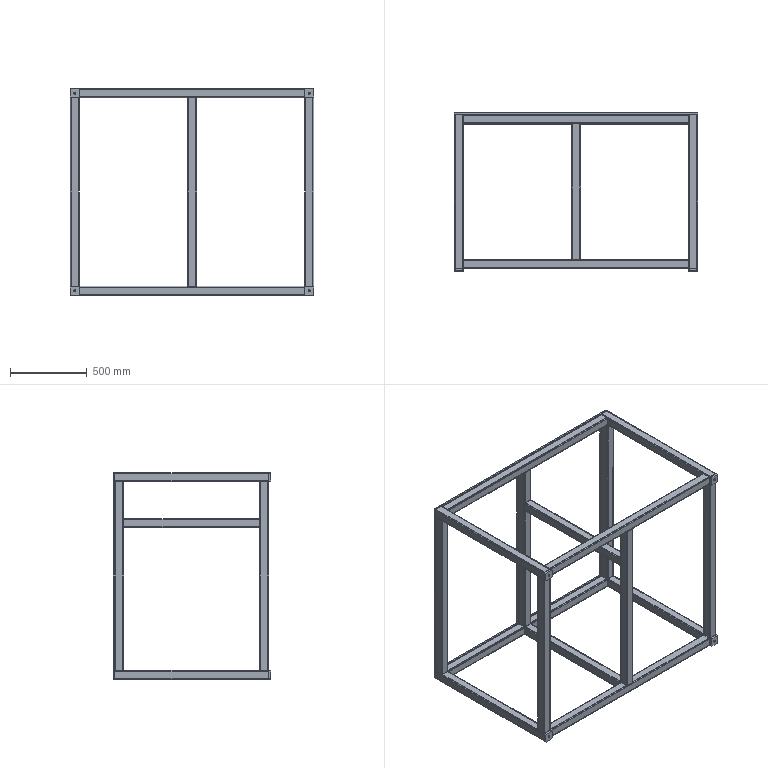Part | SolidWorks | features HoleWzd 4, ICE 3, 3DProfileFeature 1, WeldCornerFeat 1, WeldMemberFeat 1, WeldmentFeature 1 | 25 solids | 442 faces | box 1590 x 1030 x 1350 mm | volume 17668090 mm3 | plane 234 | cylinder 208 | commonest cylinder face diameters 5 x72 6.4 x64 12.8 x64 14 x8